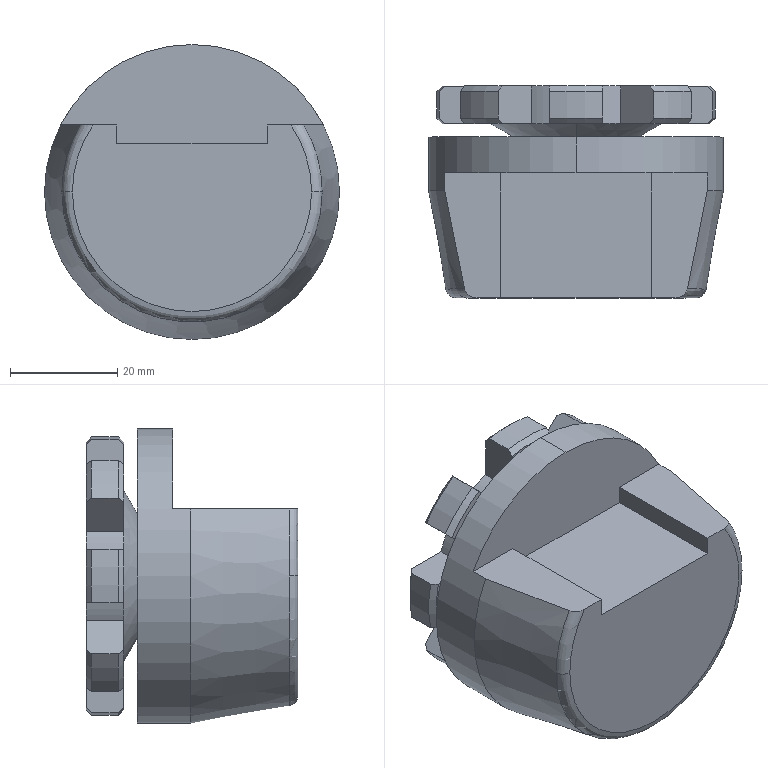Part | STEP file | HJHI_CGR51-60-U-004 | 1 solid | 77 faces | box 55 x 39.5 x 55 mm | volume 65698 mm3 | plane 28 | cylinder 23 | cone 23 | torus 3 | commonest cylinder face diameters 52 x9 35 x8 4.134 x2 10 x2 55 x2